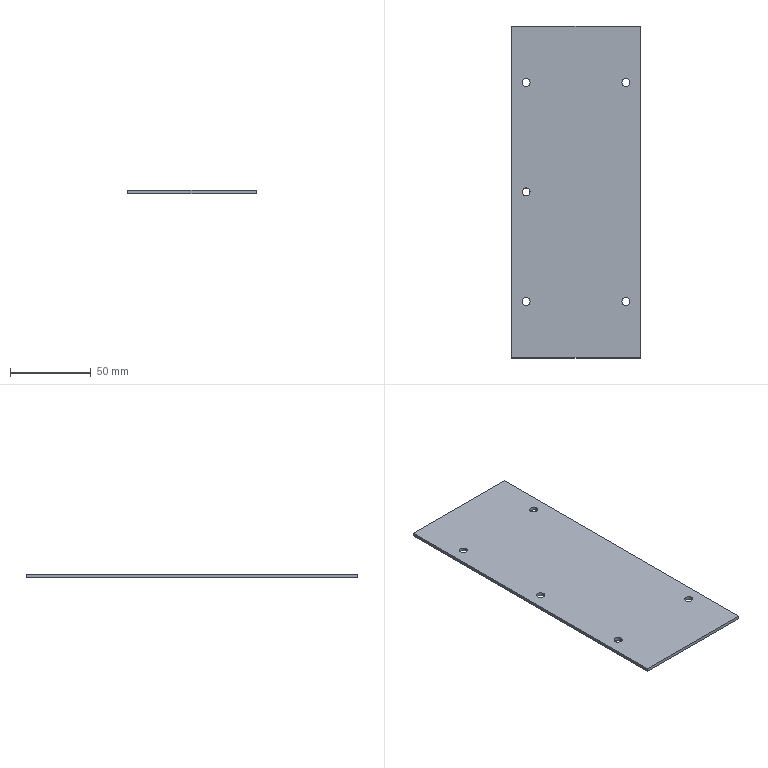Part | SolidWorks | features Extrusion 1, HoleWzd 1 | 1 solid | 16 faces | box 80 x 206 x 2 mm | volume 32764 mm3 | cylinder 10 | plane 6 | commonest cylinder face diameters 5 x10
STEP:
#1=CARTESIAN_POINT('',(28.5,68.,-1.));
#2=VERTEX_POINT('',#1);
#3=CARTESIAN_POINT('',(33.5,68.,-1.));
#4=VERTEX_POINT('',#3);
#5=CARTESIAN_POINT('',(31.,68.,-1.));
#6=DIRECTION('',(0.,0.,1.));
#7=DIRECTION('',(1.,0.,0.));
#8=AXIS2_PLACEMENT_3D('',#5,#6,#7);
#9=CIRCLE('',#8,2.5);
#10=EDGE_CURVE('',#2,#4,#9,.T.);
#11=ORIENTED_EDGE('',*,*,#10,.F.);
#12=CARTESIAN_POINT('',(28.5,68.,1.));
#13=VERTEX_POINT('',#12);
#14=CARTESIAN_POINT('',(28.5,68.,1.));
#15=DIRECTION('',(0.,0.,1.));
#16=VECTOR('',#15,1000.);
#17=LINE('',#14,#16);
#18=EDGE_CURVE('',#2,#13,#17,.T.);
#19=ORIENTED_EDGE('',*,*,#18,.T.);
#20=CARTESIAN_POINT('',(33.5,68.,1.));
#21=VERTEX_POINT('',#20);
#22=CARTESIAN_POINT('',(31.,68.,1.));
#23=DIRECTION('',(0.,0.,1.));
#24=DIRECTION('',(1.,0.,0.));
#25=AXIS2_PLACEMENT_3D('',#22,#23,#24);
#26=CIRCLE('',#25,2.5);
#27=EDGE_CURVE('',#13,#21,#26,.T.);
#28=ORIENTED_EDGE('',*,*,#27,.T.);
#29=CARTESIAN_POINT('',(33.5,68.,1.));
#30=DIRECTION('',(0.,0.,1.));
#31=VECTOR('',#30,1000.);
#32=LINE('',#29,#31);
#33=EDGE_CURVE('',#4,#21,#32,.T.);
#34=ORIENTED_EDGE('',*,*,#33,.F.);
#35=EDGE_LOOP('',(#11,#19,#28,#34));
#36=FACE_OUTER_BOUND('',#35,.T.);
#37=CARTESIAN_POINT('',(31.,68.,1.));
#38=DIRECTION('',(0.,0.,1.));
#39=DIRECTION('',(1.,0.,0.));
#40=AXIS2_PLACEMENT_3D('',#37,#38,#39);
#41=CYLINDRICAL_SURFACE('',#40,2.5);
#42=ADVANCED_FACE('',(#36),#41,.F.);
#43=CARTESIAN_POINT('',(-33.5,-68.,-1.));
#44=VERTEX_POINT('',#43);
#45=CARTESIAN_POINT('',(-28.5,-68.,-1.));
#46=VERTEX_POINT('',#45);
#47=CARTESIAN_POINT('',(-31.,-68.,-1.));
#48=DIRECTION('',(0.,0.,1.));
#49=DIRECTION('',(1.,0.,0.));
#50=AXIS2_PLACEMENT_3D('',#47,#48,#49);
#51=CIRCLE('',#50,2.5);
#52=EDGE_CURVE('',#44,#46,#51,.T.);
#53=ORIENTED_EDGE('',*,*,#52,.F.);
#54=CARTESIAN_POINT('',(-33.5,-68.,1.));
#55=VERTEX_POINT('',#54);
#56=CARTESIAN_POINT('',(-33.5,-68.,1.));
#57=DIRECTION('',(0.,0.,1.));
#58=VECTOR('',#57,1000.);
#59=LINE('',#56,#58);
#60=EDGE_CURVE('',#44,#55,#59,.T.);
#61=ORIENTED_EDGE('',*,*,#60,.T.);
#62=CARTESIAN_POINT('',(-28.5,-68.,1.));
#63=VERTEX_POINT('',#62);
#64=CARTESIAN_POINT('',(-31.,-68.,1.));
#65=DIRECTION('',(0.,0.,1.));
#66=DIRECTION('',(1.,0.,0.));
#67=AXIS2_PLACEMENT_3D('',#64,#65,#66);
#68=CIRCLE('',#67,2.5);
#69=EDGE_CURVE('',#55,#63,#68,.T.);
#70=ORIENTED_EDGE('',*,*,#69,.T.);
#71=CARTESIAN_POINT('',(-28.5,-68.,1.));
#72=DIRECTION('',(0.,0.,1.));
#73=VECTOR('',#72,1000.);
#74=LINE('',#71,#73);
#75=EDGE_CURVE('',#46,#63,#74,.T.);
#76=ORIENTED_EDGE('',*,*,#75,.F.);
#77=EDGE_LOOP('',(#53,#61,#70,#76));
#78=FACE_OUTER_BOUND('',#77,.T.);
#79=CARTESIAN_POINT('',(-31.,-68.,1.));
#80=DIRECTION('',(0.,0.,1.));
#81=DIRECTION('',(1.,0.,0.));
#82=AXIS2_PLACEMENT_3D('',#79,#80,#81);
#83=CYLINDRICAL_SURFACE('',#82,2.5);
#84=ADVANCED_FACE('',(#78),#83,.F.);
#85=CARTESIAN_POINT('',(-33.5,68.,-1.));
#86=VERTEX_POINT('',#85);
#87=CARTESIAN_POINT('',(-28.5,68.,-1.));
#88=VERTEX_POINT('',#87);
#89=CARTESIAN_POINT('',(-31.,68.,-1.));
#90=DIRECTION('',(0.,0.,1.));
#91=DIRECTION('',(1.,0.,0.));
#92=AXIS2_PLACEMENT_3D('',#89,#90,#91);
#93=CIRCLE('',#92,2.5);
#94=EDGE_CURVE('',#86,#88,#93,.T.);
#95=ORIENTED_EDGE('',*,*,#94,.F.);
#96=CARTESIAN_POINT('',(-33.5,68.,1.));
#97=VERTEX_POINT('',#96);
#98=CARTESIAN_POINT('',(-33.5,68.,1.));
#99=DIRECTION('',(0.,0.,1.));
#100=VECTOR('',#99,1000.);
#101=LINE('',#98,#100);
#102=EDGE_CURVE('',#86,#97,#101,.T.);
#103=ORIENTED_EDGE('',*,*,#102,.T.);
#104=CARTESIAN_POINT('',(-28.5,68.,1.));
#105=VERTEX_POINT('',#104);
#106=CARTESIAN_POINT('',(-31.,68.,1.));
#107=DIRECTION('',(0.,0.,1.));
#108=DIRECTION('',(1.,0.,0.));
#109=AXIS2_PLACEMENT_3D('',#106,#107,#108);
#110=CIRCLE('',#109,2.5);
#111=EDGE_CURVE('',#97,#105,#110,.T.);
#112=ORIENTED_EDGE('',*,*,#111,.T.);
#113=CARTESIAN_POINT('',(-28.5,68.,1.));
#114=DIRECTION('',(0.,0.,1.));
#115=VECTOR('',#114,1000.);
#116=LINE('',#113,#115);
#117=EDGE_CURVE('',#88,#105,#116,.T.);
#118=ORIENTED_EDGE('',*,*,#117,.F.);
#119=EDGE_LOOP('',(#95,#103,#112,#118));
#120=FACE_OUTER_BOUND('',#119,.T.);
#121=CARTESIAN_POINT('',(-31.,68.,1.));
#122=DIRECTION('',(0.,0.,1.));
#123=DIRECTION('',(1.,0.,0.));
#124=AXIS2_PLACEMENT_3D('',#121,#122,#123);
#125=CYLINDRICAL_SURFACE('',#124,2.5);
#126=ADVANCED_FACE('',(#120),#125,.F.);
#127=CARTESIAN_POINT('',(28.5,-68.,-1.));
#128=VERTEX_POINT('',#127);
#129=CARTESIAN_POINT('',(33.5,-68.,-1.));
#130=VERTEX_POINT('',#129);
#131=CARTESIAN_POINT('',(31.,-68.,-1.));
#132=DIRECTION('',(0.,0.,1.));
#133=DIRECTION('',(1.,0.,0.));
#134=AXIS2_PLACEMENT_3D('',#131,#132,#133);
#135=CIRCLE('',#134,2.5);
#136=EDGE_CURVE('',#128,#130,#135,.T.);
#137=ORIENTED_EDGE('',*,*,#136,.F.);
#138=CARTESIAN_POINT('',(28.5,-68.,1.));
#139=VERTEX_POINT('',#138);
#140=CARTESIAN_POINT('',(28.5,-68.,1.));
#141=DIRECTION('',(0.,0.,1.));
#142=VECTOR('',#141,1000.);
#143=LINE('',#140,#142);
#144=EDGE_CURVE('',#128,#139,#143,.T.);
#145=ORIENTED_EDGE('',*,*,#144,.T.);
#146=CARTESIAN_POINT('',(33.5,-68.,1.));
#147=VERTEX_POINT('',#146);
#148=CARTESIAN_POINT('',(31.,-68.,1.));
#149=DIRECTION('',(0.,0.,1.));
#150=DIRECTION('',(1.,0.,0.));
#151=AXIS2_PLACEMENT_3D('',#148,#149,#150);
#152=CIRCLE('',#151,2.5);
#153=EDGE_CURVE('',#139,#147,#152,.T.);
#154=ORIENTED_EDGE('',*,*,#153,.T.);
#155=CARTESIAN_POINT('',(33.5,-68.,1.));
#156=DIRECTION('',(0.,0.,1.));
#157=VECTOR('',#156,1000.);
#158=LINE('',#155,#157);
#159=EDGE_CURVE('',#130,#147,#158,.T.);
#160=ORIENTED_EDGE('',*,*,#159,.F.);
#161=EDGE_LOOP('',(#137,#145,#154,#160));
#162=FACE_OUTER_BOUND('',#161,.T.);
#163=CARTESIAN_POINT('',(31.,-68.,1.));
#164=DIRECTION('',(0.,0.,1.));
#165=DIRECTION('',(1.,0.,0.));
#166=AXIS2_PLACEMENT_3D('',#163,#164,#165);
#167=CYLINDRICAL_SURFACE('',#166,2.5);
#168=ADVANCED_FACE('',(#162),#167,.F.);
#169=CARTESIAN_POINT('',(-33.5,0.,-1.));
#170=VERTEX_POINT('',#169);
#171=CARTESIAN_POINT('',(-28.5,0.,-1.));
#172=VERTEX_POINT('',#171);
#173=CARTESIAN_POINT('',(-31.,0.,-1.));
#174=DIRECTION('',(0.,0.,1.));
#175=DIRECTION('',(1.,0.,0.));
#176=AXIS2_PLACEMENT_3D('',#173,#174,#175);
#177=CIRCLE('',#176,2.5);
#178=EDGE_CURVE('',#170,#172,#177,.T.);
#179=ORIENTED_EDGE('',*,*,#178,.F.);
#180=CARTESIAN_POINT('',(-33.5,0.,1.));
#181=VERTEX_POINT('',#180);
#182=CARTESIAN_POINT('',(-33.5,0.,1.));
#183=DIRECTION('',(0.,0.,1.));
#184=VECTOR('',#183,1000.);
#185=LINE('',#182,#184);
#186=EDGE_CURVE('',#170,#181,#185,.T.);
#187=ORIENTED_EDGE('',*,*,#186,.T.);
#188=CARTESIAN_POINT('',(-28.5,0.,1.));
#189=VERTEX_POINT('',#188);
#190=CARTESIAN_POINT('',(-31.,0.,1.));
#191=DIRECTION('',(0.,0.,1.));
#192=DIRECTION('',(1.,0.,0.));
#193=AXIS2_PLACEMENT_3D('',#190,#191,#192);
#194=CIRCLE('',#193,2.5);
#195=EDGE_CURVE('',#181,#189,#194,.T.);
#196=ORIENTED_EDGE('',*,*,#195,.T.);
#197=CARTESIAN_POINT('',(-28.5,0.,1.));
#198=DIRECTION('',(0.,0.,1.));
#199=VECTOR('',#198,1000.);
#200=LINE('',#197,#199);
#201=EDGE_CURVE('',#172,#189,#200,.T.);
#202=ORIENTED_EDGE('',*,*,#201,.F.);
#203=EDGE_LOOP('',(#179,#187,#196,#202));
#204=FACE_OUTER_BOUND('',#203,.T.);
#205=CARTESIAN_POINT('',(-31.,0.,1.));
#206=DIRECTION('',(0.,0.,1.));
#207=DIRECTION('',(1.,0.,0.));
#208=AXIS2_PLACEMENT_3D('',#205,#206,#207);
#209=CYLINDRICAL_SURFACE('',#208,2.5);
#210=ADVANCED_FACE('',(#204),#209,.F.);
#211=CARTESIAN_POINT('',(-40.,103.,-1.));
#212=VERTEX_POINT('',#211);
#213=CARTESIAN_POINT('',(-40.,-103.,-1.));
#214=VERTEX_POINT('',#213);
#215=CARTESIAN_POINT('',(-40.,-103.,-1.));
#216=DIRECTION('',(0.,-1.,0.));
#217=VECTOR('',#216,1000.);
#218=LINE('',#215,#217);
#219=EDGE_CURVE('',#212,#214,#218,.T.);
#220=ORIENTED_EDGE('',*,*,#219,.T.);
#221=CARTESIAN_POINT('',(-40.,-103.,1.));
#222=VERTEX_POINT('',#221);
#223=CARTESIAN_POINT('',(-40.,-103.,1.));
#224=DIRECTION('',(0.,0.,-1.));
#225=VECTOR('',#224,1000.);
#226=LINE('',#223,#225);
#227=EDGE_CURVE('',#222,#214,#226,.T.);
#228=ORIENTED_EDGE('',*,*,#227,.F.);
#229=CARTESIAN_POINT('',(-40.,103.,1.));
#230=VERTEX_POINT('',#229);
#231=CARTESIAN_POINT('',(-40.,-103.,1.));
#232=DIRECTION('',(0.,-1.,0.));
#233=VECTOR('',#232,1000.);
#234=LINE('',#231,#233);
#235=EDGE_CURVE('',#230,#222,#234,.T.);
#236=ORIENTED_EDGE('',*,*,#235,.F.);
#237=CARTESIAN_POINT('',(-40.,103.,1.));
#238=DIRECTION('',(0.,0.,-1.));
#239=VECTOR('',#238,1000.);
#240=LINE('',#237,#239);
#241=EDGE_CURVE('',#230,#212,#240,.T.);
#242=ORIENTED_EDGE('',*,*,#241,.T.);
#243=EDGE_LOOP('',(#220,#228,#236,#242));
#244=FACE_OUTER_BOUND('',#243,.T.);
#245=CARTESIAN_POINT('',(-40.,-103.,1.));
#246=DIRECTION('',(1.,0.,0.));
#247=DIRECTION('',(0.,0.,-1.));
#248=AXIS2_PLACEMENT_3D('',#245,#246,#247);
#249=PLANE('',#248);
#250=ADVANCED_FACE('',(#244),#249,.F.);
#251=CARTESIAN_POINT('',(40.,-103.,-1.));
#252=VERTEX_POINT('',#251);
#253=CARTESIAN_POINT('',(40.,-103.,-1.));
#254=DIRECTION('',(1.,0.,0.));
#255=VECTOR('',#254,1000.);
#256=LINE('',#253,#255);
#257=EDGE_CURVE('',#214,#252,#256,.T.);
#258=ORIENTED_EDGE('',*,*,#257,.T.);
#259=CARTESIAN_POINT('',(40.,-103.,1.));
#260=VERTEX_POINT('',#259);
#261=CARTESIAN_POINT('',(40.,-103.,1.));
#262=DIRECTION('',(0.,0.,-1.));
#263=VECTOR('',#262,1000.);
#264=LINE('',#261,#263);
#265=EDGE_CURVE('',#260,#252,#264,.T.);
#266=ORIENTED_EDGE('',*,*,#265,.F.);
#267=CARTESIAN_POINT('',(40.,-103.,1.));
#268=DIRECTION('',(1.,0.,0.));
#269=VECTOR('',#268,1000.);
#270=LINE('',#267,#269);
#271=EDGE_CURVE('',#222,#260,#270,.T.);
#272=ORIENTED_EDGE('',*,*,#271,.F.);
#273=ORIENTED_EDGE('',*,*,#227,.T.);
#274=EDGE_LOOP('',(#258,#266,#272,#273));
#275=FACE_OUTER_BOUND('',#274,.T.);
#276=CARTESIAN_POINT('',(40.,-103.,1.));
#277=DIRECTION('',(0.,1.,0.));
#278=DIRECTION('',(-1.,0.,0.));
#279=AXIS2_PLACEMENT_3D('',#276,#277,#278);
#280=PLANE('',#279);
#281=ADVANCED_FACE('',(#275),#280,.F.);
#282=CARTESIAN_POINT('',(40.,103.,-1.));
#283=VERTEX_POINT('',#282);
#284=CARTESIAN_POINT('',(40.,-103.,-1.));
#285=DIRECTION('',(0.,1.,0.));
#286=VECTOR('',#285,1000.);
#287=LINE('',#284,#286);
#288=EDGE_CURVE('',#252,#283,#287,.T.);
#289=ORIENTED_EDGE('',*,*,#288,.T.);
#290=CARTESIAN_POINT('',(40.,103.,1.));
#291=VERTEX_POINT('',#290);
#292=CARTESIAN_POINT('',(40.,103.,1.));
#293=DIRECTION('',(0.,0.,-1.));
#294=VECTOR('',#293,1000.);
#295=LINE('',#292,#294);
#296=EDGE_CURVE('',#291,#283,#295,.T.);
#297=ORIENTED_EDGE('',*,*,#296,.F.);
#298=CARTESIAN_POINT('',(40.,-103.,1.));
#299=DIRECTION('',(0.,1.,0.));
#300=VECTOR('',#299,1000.);
#301=LINE('',#298,#300);
#302=EDGE_CURVE('',#260,#291,#301,.T.);
#303=ORIENTED_EDGE('',*,*,#302,.F.);
#304=ORIENTED_EDGE('',*,*,#265,.T.);
#305=EDGE_LOOP('',(#289,#297,#303,#304));
#306=FACE_OUTER_BOUND('',#305,.T.);
#307=CARTESIAN_POINT('',(40.,-103.,1.));
#308=DIRECTION('',(-1.,0.,0.));
#309=DIRECTION('',(0.,0.,1.));
#310=AXIS2_PLACEMENT_3D('',#307,#308,#309);
#311=PLANE('',#310);
#312=ADVANCED_FACE('',(#306),#311,.F.);
#313=CARTESIAN_POINT('',(40.,103.,-1.));
#314=DIRECTION('',(-1.,0.,0.));
#315=VECTOR('',#314,1000.);
#316=LINE('',#313,#315);
#317=EDGE_CURVE('',#283,#212,#316,.T.);
#318=ORIENTED_EDGE('',*,*,#317,.T.);
#319=ORIENTED_EDGE('',*,*,#241,.F.);
#320=CARTESIAN_POINT('',(40.,103.,1.));
#321=DIRECTION('',(-1.,0.,0.));
#322=VECTOR('',#321,1000.);
#323=LINE('',#320,#322);
#324=EDGE_CURVE('',#291,#230,#323,.T.);
#325=ORIENTED_EDGE('',*,*,#324,.F.);
#326=ORIENTED_EDGE('',*,*,#296,.T.);
#327=EDGE_LOOP('',(#318,#319,#325,#326));
#328=FACE_OUTER_BOUND('',#327,.T.);
#329=CARTESIAN_POINT('',(40.,103.,1.));
#330=DIRECTION('',(0.,-1.,0.));
#331=DIRECTION('',(0.,0.,-1.));
#332=AXIS2_PLACEMENT_3D('',#329,#330,#331);
#333=PLANE('',#332);
#334=ADVANCED_FACE('',(#328),#333,.F.);
#335=CARTESIAN_POINT('',(31.,68.,1.));
#336=DIRECTION('',(0.,0.,1.));
#337=DIRECTION('',(1.,0.,0.));
#338=AXIS2_PLACEMENT_3D('',#335,#336,#337);
#339=CIRCLE('',#338,2.5);
#340=EDGE_CURVE('',#21,#13,#339,.T.);
#341=ORIENTED_EDGE('',*,*,#340,.F.);
#342=ORIENTED_EDGE('',*,*,#27,.F.);
#343=EDGE_LOOP('',(#341,#342));
#344=FACE_BOUND('',#343,.T.);
#345=CARTESIAN_POINT('',(-31.,-68.,1.));
#346=DIRECTION('',(0.,0.,1.));
#347=DIRECTION('',(1.,0.,0.));
#348=AXIS2_PLACEMENT_3D('',#345,#346,#347);
#349=CIRCLE('',#348,2.5);
#350=EDGE_CURVE('',#63,#55,#349,.T.);
#351=ORIENTED_EDGE('',*,*,#350,.F.);
#352=ORIENTED_EDGE('',*,*,#69,.F.);
#353=EDGE_LOOP('',(#351,#352));
#354=FACE_BOUND('',#353,.T.);
#355=CARTESIAN_POINT('',(-31.,68.,1.));
#356=DIRECTION('',(0.,0.,1.));
#357=DIRECTION('',(1.,0.,0.));
#358=AXIS2_PLACEMENT_3D('',#355,#356,#357);
#359=CIRCLE('',#358,2.5);
#360=EDGE_CURVE('',#105,#97,#359,.T.);
#361=ORIENTED_EDGE('',*,*,#360,.F.);
#362=ORIENTED_EDGE('',*,*,#111,.F.);
#363=EDGE_LOOP('',(#361,#362));
#364=FACE_BOUND('',#363,.T.);
#365=CARTESIAN_POINT('',(31.,-68.,1.));
#366=DIRECTION('',(0.,0.,1.));
#367=DIRECTION('',(1.,0.,0.));
#368=AXIS2_PLACEMENT_3D('',#365,#366,#367);
#369=CIRCLE('',#368,2.5);
#370=EDGE_CURVE('',#147,#139,#369,.T.);
#371=ORIENTED_EDGE('',*,*,#370,.F.);
#372=ORIENTED_EDGE('',*,*,#153,.F.);
#373=EDGE_LOOP('',(#371,#372));
#374=FACE_BOUND('',#373,.T.);
#375=CARTESIAN_POINT('',(-31.,0.,1.));
#376=DIRECTION('',(0.,0.,1.));
#377=DIRECTION('',(1.,0.,0.));
#378=AXIS2_PLACEMENT_3D('',#375,#376,#377);
#379=CIRCLE('',#378,2.5);
#380=EDGE_CURVE('',#189,#181,#379,.T.);
#381=ORIENTED_EDGE('',*,*,#380,.F.);
#382=ORIENTED_EDGE('',*,*,#195,.F.);
#383=EDGE_LOOP('',(#381,#382));
#384=FACE_BOUND('',#383,.T.);
#385=ORIENTED_EDGE('',*,*,#235,.T.);
#386=ORIENTED_EDGE('',*,*,#271,.T.);
#387=ORIENTED_EDGE('',*,*,#302,.T.);
#388=ORIENTED_EDGE('',*,*,#324,.T.);
#389=EDGE_LOOP('',(#385,#386,#387,#388));
#390=FACE_OUTER_BOUND('',#389,.T.);
#391=CARTESIAN_POINT('',(0.,0.,1.));
#392=DIRECTION('',(0.,0.,1.));
#393=DIRECTION('',(1.,0.,0.));
#394=AXIS2_PLACEMENT_3D('',#391,#392,#393);
#395=PLANE('',#394);
#396=ADVANCED_FACE('',(#344,#354,#364,#374,#384,#390),#395,.T.);
#397=CARTESIAN_POINT('',(31.,68.,-1.));
#398=DIRECTION('',(0.,0.,1.));
#399=DIRECTION('',(1.,0.,0.));
#400=AXIS2_PLACEMENT_3D('',#397,#398,#399);
#401=CIRCLE('',#400,2.5);
#402=EDGE_CURVE('',#4,#2,#401,.T.);
#403=ORIENTED_EDGE('',*,*,#402,.T.);
#404=ORIENTED_EDGE('',*,*,#10,.T.);
#405=EDGE_LOOP('',(#403,#404));
#406=FACE_BOUND('',#405,.T.);
#407=CARTESIAN_POINT('',(-31.,-68.,-1.));
#408=DIRECTION('',(0.,0.,1.));
#409=DIRECTION('',(1.,0.,0.));
#410=AXIS2_PLACEMENT_3D('',#407,#408,#409);
#411=CIRCLE('',#410,2.5);
#412=EDGE_CURVE('',#46,#44,#411,.T.);
#413=ORIENTED_EDGE('',*,*,#412,.T.);
#414=ORIENTED_EDGE('',*,*,#52,.T.);
#415=EDGE_LOOP('',(#413,#414));
#416=FACE_BOUND('',#415,.T.);
#417=CARTESIAN_POINT('',(-31.,68.,-1.));
#418=DIRECTION('',(0.,0.,1.));
#419=DIRECTION('',(1.,0.,0.));
#420=AXIS2_PLACEMENT_3D('',#417,#418,#419);
#421=CIRCLE('',#420,2.5);
#422=EDGE_CURVE('',#88,#86,#421,.T.);
#423=ORIENTED_EDGE('',*,*,#422,.T.);
#424=ORIENTED_EDGE('',*,*,#94,.T.);
#425=EDGE_LOOP('',(#423,#424));
#426=FACE_BOUND('',#425,.T.);
#427=CARTESIAN_POINT('',(31.,-68.,-1.));
#428=DIRECTION('',(0.,0.,1.));
#429=DIRECTION('',(1.,0.,0.));
#430=AXIS2_PLACEMENT_3D('',#427,#428,#429);
#431=CIRCLE('',#430,2.5);
#432=EDGE_CURVE('',#130,#128,#431,.T.);
#433=ORIENTED_EDGE('',*,*,#432,.T.);
#434=ORIENTED_EDGE('',*,*,#136,.T.);
#435=EDGE_LOOP('',(#433,#434));
#436=FACE_BOUND('',#435,.T.);
#437=CARTESIAN_POINT('',(-31.,0.,-1.));
#438=DIRECTION('',(0.,0.,1.));
#439=DIRECTION('',(1.,0.,0.));
#440=AXIS2_PLACEMENT_3D('',#437,#438,#439);
#441=CIRCLE('',#440,2.5);
#442=EDGE_CURVE('',#172,#170,#441,.T.);
#443=ORIENTED_EDGE('',*,*,#442,.T.);
#444=ORIENTED_EDGE('',*,*,#178,.T.);
#445=EDGE_LOOP('',(#443,#444));
#446=FACE_BOUND('',#445,.T.);
#447=ORIENTED_EDGE('',*,*,#219,.F.);
#448=ORIENTED_EDGE('',*,*,#317,.F.);
#449=ORIENTED_EDGE('',*,*,#288,.F.);
#450=ORIENTED_EDGE('',*,*,#257,.F.);
#451=EDGE_LOOP('',(#447,#448,#449,#450));
#452=FACE_OUTER_BOUND('',#451,.T.);
#453=CARTESIAN_POINT('',(0.,0.,-1.));
#454=DIRECTION('',(0.,0.,1.));
#455=DIRECTION('',(1.,0.,0.));
#456=AXIS2_PLACEMENT_3D('',#453,#454,#455);
#457=PLANE('',#456);
#458=ADVANCED_FACE('',(#406,#416,#426,#436,#446,#452),#457,.F.);
#459=ORIENTED_EDGE('',*,*,#186,.F.);
#460=ORIENTED_EDGE('',*,*,#442,.F.);
#461=ORIENTED_EDGE('',*,*,#201,.T.);
#462=ORIENTED_EDGE('',*,*,#380,.T.);
#463=EDGE_LOOP('',(#459,#460,#461,#462));
#464=FACE_OUTER_BOUND('',#463,.T.);
#465=CARTESIAN_POINT('',(-31.,0.,1.));
#466=DIRECTION('',(0.,0.,1.));
#467=DIRECTION('',(1.,0.,0.));
#468=AXIS2_PLACEMENT_3D('',#465,#466,#467);
#469=CYLINDRICAL_SURFACE('',#468,2.5);
#470=ADVANCED_FACE('',(#464),#469,.F.);
#471=ORIENTED_EDGE('',*,*,#144,.F.);
#472=ORIENTED_EDGE('',*,*,#432,.F.);
#473=ORIENTED_EDGE('',*,*,#159,.T.);
#474=ORIENTED_EDGE('',*,*,#370,.T.);
#475=EDGE_LOOP('',(#471,#472,#473,#474));
#476=FACE_OUTER_BOUND('',#475,.T.);
#477=CARTESIAN_POINT('',(31.,-68.,1.));
#478=DIRECTION('',(0.,0.,1.));
#479=DIRECTION('',(1.,0.,0.));
#480=AXIS2_PLACEMENT_3D('',#477,#478,#479);
#481=CYLINDRICAL_SURFACE('',#480,2.5);
#482=ADVANCED_FACE('',(#476),#481,.F.);
#483=ORIENTED_EDGE('',*,*,#102,.F.);
#484=ORIENTED_EDGE('',*,*,#422,.F.);
#485=ORIENTED_EDGE('',*,*,#117,.T.);
#486=ORIENTED_EDGE('',*,*,#360,.T.);
#487=EDGE_LOOP('',(#483,#484,#485,#486));
#488=FACE_OUTER_BOUND('',#487,.T.);
#489=CARTESIAN_POINT('',(-31.,68.,1.));
#490=DIRECTION('',(0.,0.,1.));
#491=DIRECTION('',(1.,0.,0.));
#492=AXIS2_PLACEMENT_3D('',#489,#490,#491);
#493=CYLINDRICAL_SURFACE('',#492,2.5);
#494=ADVANCED_FACE('',(#488),#493,.F.);
#495=ORIENTED_EDGE('',*,*,#60,.F.);
#496=ORIENTED_EDGE('',*,*,#412,.F.);
#497=ORIENTED_EDGE('',*,*,#75,.T.);
#498=ORIENTED_EDGE('',*,*,#350,.T.);
#499=EDGE_LOOP('',(#495,#496,#497,#498));
#500=FACE_OUTER_BOUND('',#499,.T.);
#501=CARTESIAN_POINT('',(-31.,-68.,1.));
#502=DIRECTION('',(0.,0.,1.));
#503=DIRECTION('',(1.,0.,0.));
#504=AXIS2_PLACEMENT_3D('',#501,#502,#503);
#505=CYLINDRICAL_SURFACE('',#504,2.5);
#506=ADVANCED_FACE('',(#500),#505,.F.);
#507=ORIENTED_EDGE('',*,*,#18,.F.);
#508=ORIENTED_EDGE('',*,*,#402,.F.);
#509=ORIENTED_EDGE('',*,*,#33,.T.);
#510=ORIENTED_EDGE('',*,*,#340,.T.);
#511=EDGE_LOOP('',(#507,#508,#509,#510));
#512=FACE_OUTER_BOUND('',#511,.T.);
#513=CARTESIAN_POINT('',(31.,68.,1.));
#514=DIRECTION('',(0.,0.,1.));
#515=DIRECTION('',(1.,0.,0.));
#516=AXIS2_PLACEMENT_3D('',#513,#514,#515);
#517=CYLINDRICAL_SURFACE('',#516,2.5);
#518=ADVANCED_FACE('',(#512),#517,.F.);
#519=CLOSED_SHELL('',(#42,#84,#126,#168,#210,#250,#281,#312,#334,#396,#458,#470,#482,#494,#506,#518));
#520=MANIFOLD_SOLID_BREP('',#519);
#521=CARTESIAN_POINT('',(0.,0.,0.));
#522=DIRECTION('',(0.,0.,1.));
#523=DIRECTION('',(1.,0.,0.));
#524=AXIS2_PLACEMENT_3D('',#521,#522,#523);
#525=(LENGTH_UNIT()NAMED_UNIT(*)SI_UNIT(.MILLI.,.METRE.));
#526=UNCERTAINTY_MEASURE_WITH_UNIT(LENGTH_MEASURE(0.00001),#525,'','');
#527=(NAMED_UNIT(*)PLANE_ANGLE_UNIT()SI_UNIT($,.RADIAN.));
#528=(NAMED_UNIT(*)SI_UNIT($,.STERADIAN.)SOLID_ANGLE_UNIT());
#529=(GEOMETRIC_REPRESENTATION_CONTEXT(3)GLOBAL_UNCERTAINTY_ASSIGNED_CONTEXT((#526))GLOBAL_UNIT_ASSIGNED_CONTEXT((#525,#527,#528))REPRESENTATION_CONTEXT('',''));
#530=ADVANCED_BREP_SHAPE_REPRESENTATION('',(#520,#524),#529);